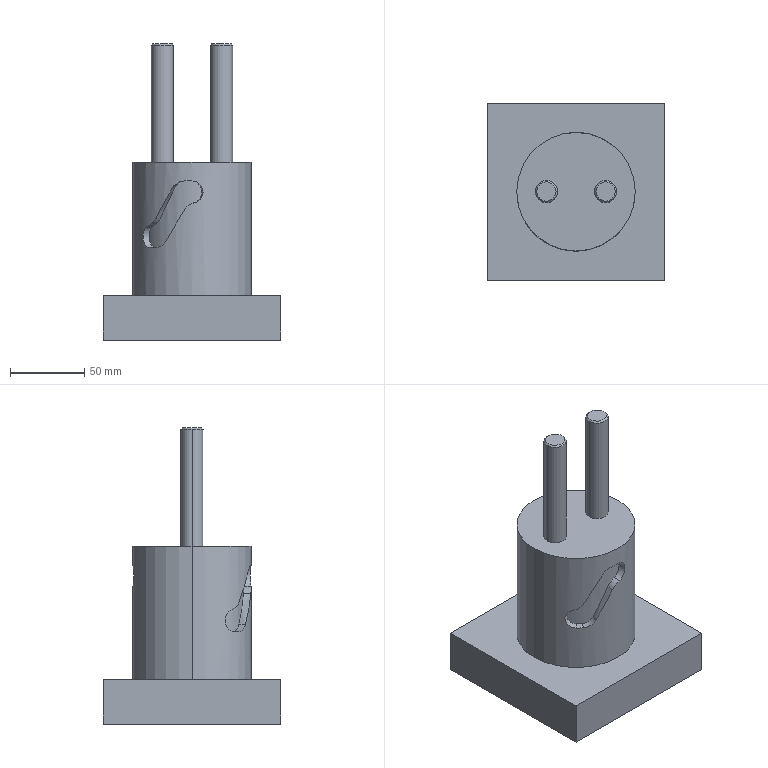Part | SolidWorks | features ICE 3, Chamfer 2, CirPattern 1, Emboss 1, Extrusion 1 | 3 solids | 49 faces | box 120 x 120 x 200 mm | volume 904225 mm3 | plane 17 | spline 16 | cylinder 12 | cone 4 | commonest cylinder face diameters 15 x8 70 x2 80 x2